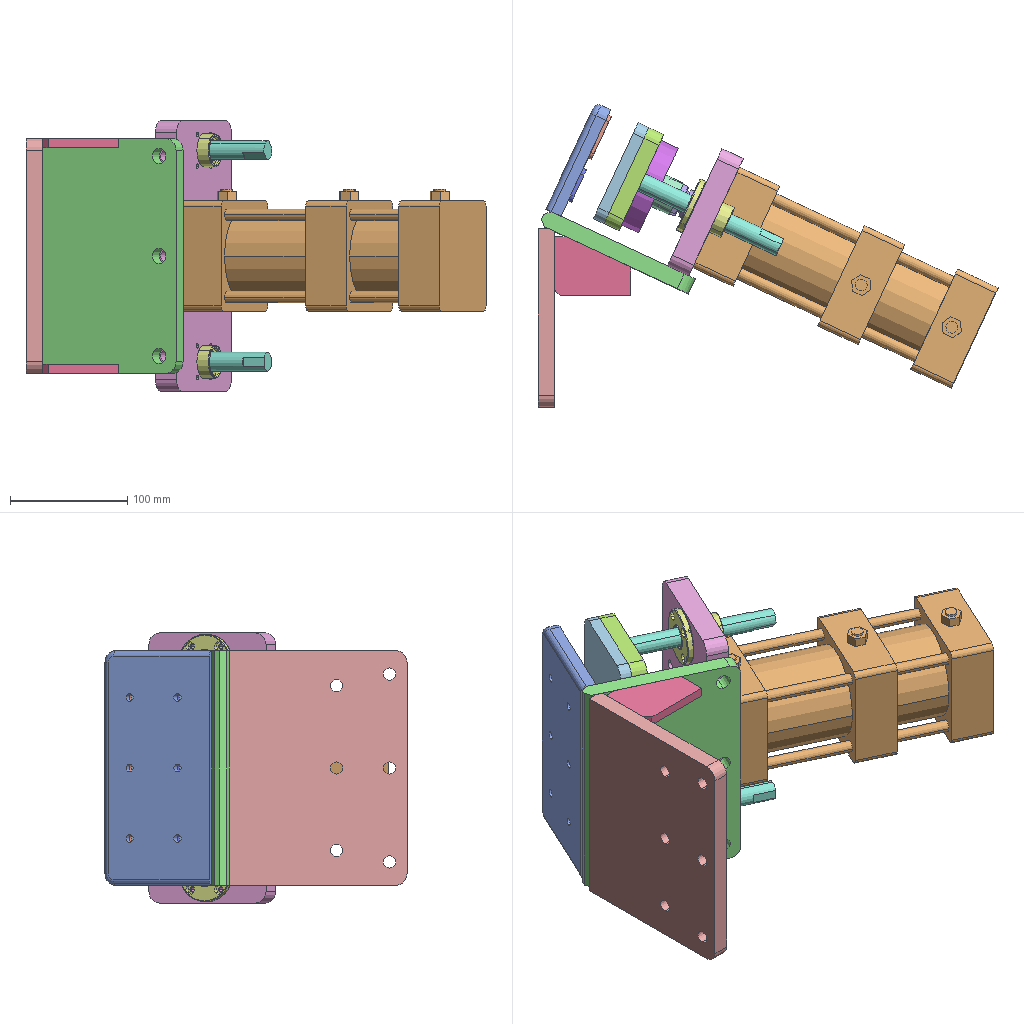Assembly | SolidWorks | 17 different items | 20 placed | box 392 x 257 x 230 mm
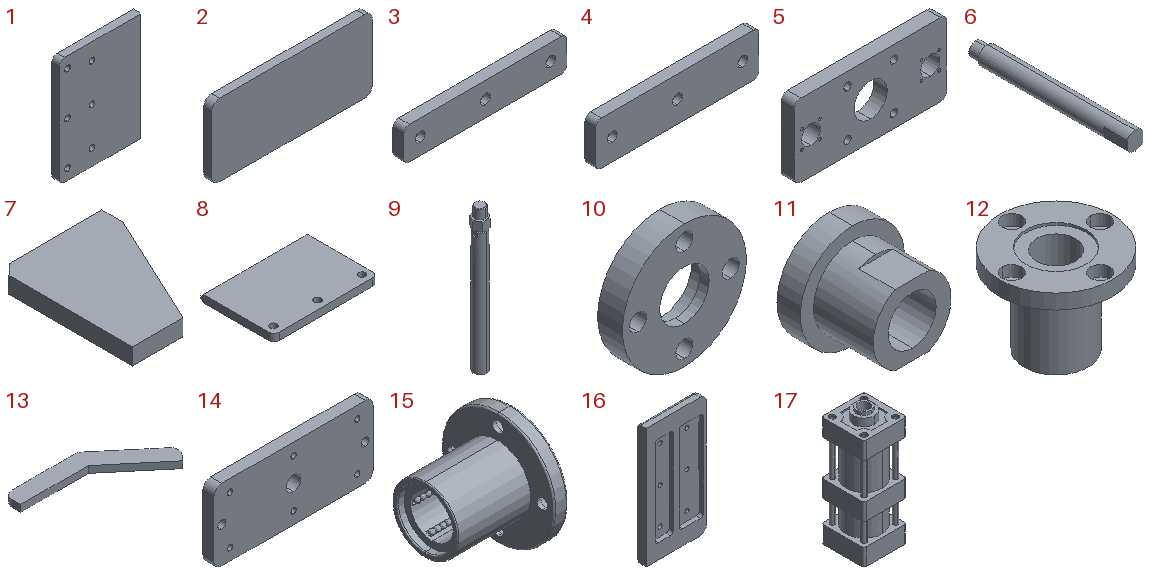Parts list (item | quantity | size | volume | features):
1 | x1 | 151.5 x 14 x 200 mm | 415411 mm3 | features HoleWzd 2, ICE 2, Extrusion 1, Fillet 1
2 | x1 | 200 x 10 x 90 mm | 179142 mm3 | features Extrusion 1, Fillet 1
3 | x1 | 150 x 10 x 30 mm | 41843 mm3 | features LPattern 2, Extrusion 1, Fillet 1, HoleWzd 1, ICE 1
4 | x1 | 150 x 10 x 40 mm | 56843 mm3 | features LPattern 2, Extrusion 1, Fillet 1, HoleWzd 1, ICE 1
5 | x1 | 230 x 20 x 110 mm | 424729 mm3 | features ICE 3, HoleWzd 2, LPattern 2, Extrusion 1, Fillet 1
6 | x2 | 16 x 140 x 16 mm | 27060 mm3 | features ICE 2, Extrusion 1, HoleWzd 1
7 | x2 | 50 x 65 x 8 mm | 20258 mm3 | features Chamfer 1, Extrusion 1
8 | x1 | 200 x 140 x 14 mm | 380824 mm3 | features ICE 2, Chamfer 1, Extrusion 1, Fillet 1
9 | x1 | 30 x 25.981 x 280 mm | 135007 mm3 | features ICE 4, Chamfer 1, Revolution 1
10 | x1 | 80 x 16 x 80 mm | 55663 mm3 | features Extrusion 1, HoleWzd 1, ICE 1
11 | x1 | 40 x 32 x 40 mm | 18596 mm3 | features ICE 2, Extrusion 1, HoleWzd 1
12 | x1 | 46 x 46 x 36 mm | 17134 mm3 | features BaseBody 1
13 | x1 | 150.051 x 71.423 x 8 mm | 26409 mm3 | features Extrusion 1, Fillet 1
14 | x1 | 200 x 14 x 90 mm | 241696 mm3 | features HoleWzd 4, Extrusion 1, Fillet 1
15 | x2 | 37 x 48 x 48 mm | 18661 mm3 | features BaseBody 1
16 | x1 | 100 x 14 x 200 mm | 202593 mm3 | features ICE 8, Fillet 3, HoleWzd 2, Chamfer 1, Extrusion 1, LPattern 1
17 | x1 | 104 x 94 x 264 mm | 1602001 mm3 | features ICE 9, Fillet 1, Revolution 1
Mates (type | each side: item.copy, entity, surface, feature):
Coincident | 8.1 face plane Boss-Extrude1 | 16.1 face plane Boss-Extrude1
Width | 1.1 face plane Boss-Extrude1 | 1.1 face plane Boss-Extrude1 | 16.1 face plane Boss-Extrude1 | 16.1 face plane Boss-Extrude1
Coincident | 5.1 face plane Boss-Extrude1 | 12.1 face
Concentric | 5.1 face cylinder Cut-Extrude2 | 12.1 face
Concentric | 5.1 face cylinder Cut-Extrude3 | 12.1 face | 2 times
Coincident | 5.1 face plane Boss-Extrude1 | 12.2 face
Concentric | 5.1 face cylinder Cut-Extrude2 | 12.2 face
Concentric | 5.1 face cylinder LPattern1 | 12.2 face
Concentric | 5.1 face | assembly face | 4 times
Coincident | 5.1 face plane Boss-Extrude1 | assembly face | 2 times
Concentric | 12.1 face | 6.1 face cylinder Boss-Extrude1
Concentric | 12.2 face | 6.2 face cylinder Boss-Extrude1
Coincident | 14.1 face plane Boss-Extrude1 | 6.1 face plane Boss-Extrude1
Coincident | 14.1 face plane Boss-Extrude1 | 6.2 face plane Boss-Extrude1
Concentric | 14.1 face cylinder M12 Tapped Hole1 | 6.1 face cylinder Boss-Extrude1
Concentric | 14.1 face cylinder M12 Tapped Hole1 | 6.2 face cylinder Boss-Extrude1
Width | 14.1 face plane Boss-Extrude1 | 14.1 face plane Boss-Extrude1 | 16.1 face plane Boss-Extrude1 | 16.1 face plane Boss-Extrude1
Coincident | 16.1 face plane Boss-Extrude1 | 14.1 face plane Boss-Extrude1
DistanceDim | 16.1 face plane Boss-Extrude1 | 5.1 face plane Boss-Extrude1
Coincident | 5.1 face plane Boss-Extrude1 | 17.1 face plane Revolve1
Concentric | 5.1 face cylinder Cut-Extrude4 | 17.1 face cylinder Revolve1
Concentric | 5.1 face cylinder Cut-Extrude4 | 17.1 face cylinder Cut-Extrude7
Concentric | 17.1 face cylinder Revolve1 | 9.1 face cylinder Revolve1
LimitDistanceDim | 9.1 face plane Cut-Extrude4 | 17.1 face plane Revolve1
DistanceDim | 14.1 face plane Boss-Extrude1 | 9.1 face plane Revolve1
Coincident | 1.1 face plane Boss-Extrude1 | assembly face | 2 times
Coincident | 16.1 face plane Boss-Extrude1 | assembly face | 2 times
Coincident | 7.1 face | 1.1 face plane Boss-Extrude1
Coincident | 16.1 face plane Boss-Extrude1 | 7.1 face | 2 times
Coincident | 7.1 face | 7.2 face | 2 times
Coincident | 1.1 face plane Boss-Extrude1 | 7.2 face
Coincident | 1.1 face plane Boss-Extrude1 | 13.1 face | 2 times
DistanceDim | 13.1 face | 1.1 face
Coincident | 1.1 face plane Boss-Extrude1 | 13.2 face
Coincident | 13.1 face | 13.2 face | 2 times
DistanceDim | 16.1 face plane Boss-Extrude1 | 8.1 face plane Boss-Extrude1
Coincident | 1.1 face plane Boss-Extrude1 | 7.3 face plane Boss-Extrude1 | 2 times
Coincident | 8.1 face plane Boss-Extrude1 | 7.4 face plane Boss-Extrude1
Coincident | 1.1 face plane Boss-Extrude1 | 7.4 face plane Boss-Extrude1
Coincident | 7.3 face plane Boss-Extrude1 | 7.4 face plane Boss-Extrude1
Coincident | 14.1 face plane Boss-Extrude1 | 2.1 face plane Boss-Extrude1 | 3 times
Coincident | 2.1 face plane Boss-Extrude1 | assembly face | 2 times
Coincident | 16.1 face plane Boss-Extrude1 | 4.1 face | 3 times
Coincident | 16.1 face plane Boss-Extrude1 | 8.1 face plane Boss-Extrude1
Coincident | 1.1 face plane Cut-Extrude1 | 8.1 face plane Boss-Extrude1
DistanceDim | 1.1 face plane Boss-Extrude1 | 8.1 edge
Coincident | 8.1 face plane Boss-Extrude1 | 7.3 face plane Boss-Extrude1
Coincident | 5.1 face plane Boss-Extrude1 | 15.1 face plane Import1
Concentric | 5.1 face cylinder Cut-Extrude2 | 15.1 face cylinder Import1
Coincident | 5.1 face plane Boss-Extrude1 | 8.1 face plane Boss-Extrude1
Concentric | 5.1 face cylinder Cut-Extrude3 | 15.1 face cylinder Import1
Coincident | 5.1 face plane Boss-Extrude1 | 15.2 face plane Import1
Concentric | 5.1 face cylinder Cut-Extrude2 | 15.2 face cylinder Import1
Concentric | 5.1 face cylinder LPattern1 | 15.2 face cylinder Import1
Coincident | 14.1 face plane Boss-Extrude1 | 10.1 face plane Boss-Extrude1
Concentric | 9.1 face cylinder Revolve1 | 10.1 face cylinder Boss-Extrude1
Coincident | 10.1 face plane Cut-Extrude1 | 11.1 face plane Cut-Extrude1
Concentric | 10.1 face cylinder Boss-Extrude1 | 11.1 face cylinder Cut-Extrude1
DistanceDim | 5.1 face plane Boss-Extrude1 | 8.1 face plane Boss-Extrude1
Coincident | 16.1 face plane Cut-Extrude6 | 4.2 face plane Boss-Extrude1
Concentric | 16.1 face cylinder M8 Tapped Hole2 | 4.2 face cylinder Socket Button Head Screw Hole1 | 2 times
Coincident | 16.1 face plane Cut-Extrude6 | 3.1 face plane Boss-Extrude1 | 3 times